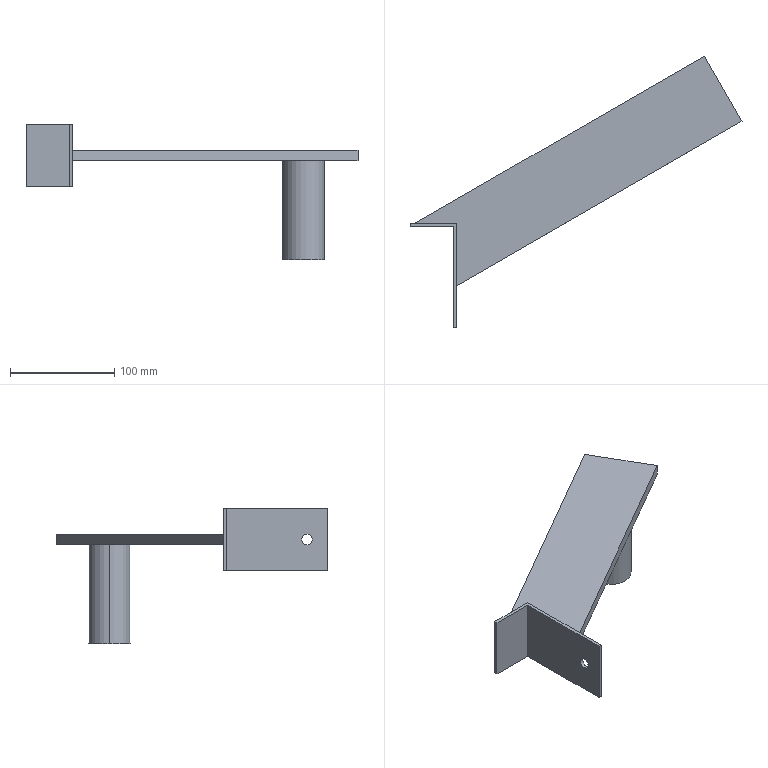Part | STEP file | 1 solid | 18 faces | box 318.145 x 260.315 x 130 mm | volume 361674 mm3 | plane 14 | cylinder 4 | commonest cylinder face diameters 10 x2 40 x2
STEP:
#1=CARTESIAN_POINT('',(0.,0.,0.));
#2=DIRECTION('',(0.,0.,1.));
#3=DIRECTION('',(1.,0.,0.));
#4=AXIS2_PLACEMENT_3D('',#1,#2,#3);
#5=CARTESIAN_POINT('',(51.255,-50.39,5.));
#6=VERTEX_POINT('',#5);
#7=CARTESIAN_POINT('',(48.255,-50.39,5.));
#8=VERTEX_POINT('',#7);
#9=CARTESIAN_POINT('',(51.255,-50.39,5.));
#10=DIRECTION('',(-1.,0.,0.));
#11=VECTOR('',#10,1.);
#12=LINE('',#9,#11);
#13=CARTESIAN_POINT('',(51.255,-50.39,0.));
#14=DIRECTION('',(-1.,0.,0.));
#15=DIRECTION('',(0.,0.,1.));
#16=AXIS2_PLACEMENT_3D('',#13,#14,#15);
#17=CYLINDRICAL_SURFACE('',#16,5.);
#18=CARTESIAN_POINT('',(6.283,0.));
#19=DIRECTION('',(0.,1.));
#20=VECTOR('',#19,1.);
#21=LINE('',#18,#20);
#22=(GEOMETRIC_REPRESENTATION_CONTEXT(2)PARAMETRIC_REPRESENTATION_CONTEXT()REPRESENTATION_CONTEXT('',''));
#23=DEFINITIONAL_REPRESENTATION('',(#21),#22);
#24=PCURVE('',#17,#23);
#25=CARTESIAN_POINT('',(51.255,-50.39,0.));
#26=DIRECTION('',(-1.,0.,0.));
#27=DIRECTION('',(0.,0.,1.));
#28=AXIS2_PLACEMENT_3D('',#25,#26,#27);
#29=CYLINDRICAL_SURFACE('',#28,5.);
#30=CARTESIAN_POINT('',(0.,0.));
#31=DIRECTION('',(0.,1.));
#32=VECTOR('',#31,1.);
#33=LINE('',#30,#32);
#34=(GEOMETRIC_REPRESENTATION_CONTEXT(2)PARAMETRIC_REPRESENTATION_CONTEXT()REPRESENTATION_CONTEXT('',''));
#35=DEFINITIONAL_REPRESENTATION('',(#33),#34);
#36=PCURVE('',#29,#35);
#37=SURFACE_CURVE('',#12,(#24,#36),.PCURVE_S1.);
#38=EDGE_CURVE('',#6,#8,#37,.T.);
#39=ORIENTED_EDGE('',*,*,#38,.T.);
#40=CARTESIAN_POINT('',(48.255,-50.39,-5.));
#41=VERTEX_POINT('',#40);
#42=CARTESIAN_POINT('',(48.255,-50.39,0.));
#43=DIRECTION('',(1.,0.,0.));
#44=DIRECTION('',(0.,0.,1.));
#45=AXIS2_PLACEMENT_3D('',#42,#43,#44);
#46=CIRCLE('',#45,5.);
#47=CARTESIAN_POINT('',(6.283,3.));
#48=DIRECTION('',(-1.,0.));
#49=VECTOR('',#48,1.);
#50=LINE('',#47,#49);
#51=(GEOMETRIC_REPRESENTATION_CONTEXT(2)PARAMETRIC_REPRESENTATION_CONTEXT()REPRESENTATION_CONTEXT('',''));
#52=DEFINITIONAL_REPRESENTATION('',(#50),#51);
#53=PCURVE('',#17,#52);
#54=CARTESIAN_POINT('',(48.255,26.61,0.));
#55=DIRECTION('',(1.,0.,0.));
#56=DIRECTION('',(0.,1.,0.));
#57=AXIS2_PLACEMENT_3D('',#54,#55,#56);
#58=PLANE('',#57);
#59=CARTESIAN_POINT('',(-77.,0.));
#60=DIRECTION('',(0.,1.));
#61=AXIS2_PLACEMENT_2D('',#59,#60);
#62=CIRCLE('',#61,5.);
#63=(GEOMETRIC_REPRESENTATION_CONTEXT(2)PARAMETRIC_REPRESENTATION_CONTEXT()REPRESENTATION_CONTEXT('',''));
#64=DEFINITIONAL_REPRESENTATION('',(#62),#63);
#65=PCURVE('',#58,#64);
#66=SURFACE_CURVE('',#46,(#53,#65),.PCURVE_S1.);
#67=EDGE_CURVE('',#8,#41,#66,.T.);
#68=ORIENTED_EDGE('',*,*,#67,.T.);
#69=CARTESIAN_POINT('',(51.255,-50.39,-5.));
#70=VERTEX_POINT('',#69);
#71=CARTESIAN_POINT('',(51.255,-50.39,-5.));
#72=DIRECTION('',(-1.,0.,0.));
#73=VECTOR('',#72,1.);
#74=LINE('',#71,#73);
#75=CARTESIAN_POINT('',(3.142,0.));
#76=DIRECTION('',(0.,1.));
#77=VECTOR('',#76,1.);
#78=LINE('',#75,#77);
#79=(GEOMETRIC_REPRESENTATION_CONTEXT(2)PARAMETRIC_REPRESENTATION_CONTEXT()REPRESENTATION_CONTEXT('',''));
#80=DEFINITIONAL_REPRESENTATION('',(#78),#79);
#81=PCURVE('',#17,#80);
#82=CARTESIAN_POINT('',(3.142,0.));
#83=DIRECTION('',(0.,1.));
#84=VECTOR('',#83,1.);
#85=LINE('',#82,#84);
#86=(GEOMETRIC_REPRESENTATION_CONTEXT(2)PARAMETRIC_REPRESENTATION_CONTEXT()REPRESENTATION_CONTEXT('',''));
#87=DEFINITIONAL_REPRESENTATION('',(#85),#86);
#88=PCURVE('',#29,#87);
#89=SURFACE_CURVE('',#74,(#81,#88),.PCURVE_S1.);
#90=EDGE_CURVE('',#70,#41,#89,.T.);
#91=ORIENTED_EDGE('',*,*,#90,.F.);
#92=CARTESIAN_POINT('',(51.255,-50.39,0.));
#93=DIRECTION('',(1.,0.,0.));
#94=DIRECTION('',(0.,0.,1.));
#95=AXIS2_PLACEMENT_3D('',#92,#93,#94);
#96=CIRCLE('',#95,5.);
#97=CARTESIAN_POINT('',(6.283,0.));
#98=DIRECTION('',(-1.,0.));
#99=VECTOR('',#98,1.);
#100=LINE('',#97,#99);
#101=(GEOMETRIC_REPRESENTATION_CONTEXT(2)PARAMETRIC_REPRESENTATION_CONTEXT()REPRESENTATION_CONTEXT('',''));
#102=DEFINITIONAL_REPRESENTATION('',(#100),#101);
#103=PCURVE('',#17,#102);
#104=CARTESIAN_POINT('',(51.255,-30.39,0.));
#105=DIRECTION('',(-1.,0.,0.));
#106=DIRECTION('',(0.,0.,1.));
#107=AXIS2_PLACEMENT_3D('',#104,#105,#106);
#108=PLANE('',#107);
#109=CARTESIAN_POINT('',(5.,-20.));
#110=CARTESIAN_POINT('',(5.,-28.66));
#111=CARTESIAN_POINT('',(-2.5,-24.33));
#112=CARTESIAN_POINT('',(-10.,-20.));
#113=CARTESIAN_POINT('',(-2.5,-15.67));
#114=CARTESIAN_POINT('',(5.,-11.34));
#115=CARTESIAN_POINT('',(5.,-20.));
#116=(BOUNDED_CURVE()B_SPLINE_CURVE(2,(#109,#110,#111,#112,#113,#114,#115),.UNSPECIFIED.,.T.,.F.)B_SPLINE_CURVE_WITH_KNOTS((1,2,2,2,2,1),(-2.094,0.,2.094,4.189,6.283,8.378),.UNSPECIFIED.)CURVE()GEOMETRIC_REPRESENTATION_ITEM()RATIONAL_B_SPLINE_CURVE((1.,0.5,1.,0.5,1.,0.5,1.))REPRESENTATION_ITEM(''));
#117=(GEOMETRIC_REPRESENTATION_CONTEXT(2)PARAMETRIC_REPRESENTATION_CONTEXT()REPRESENTATION_CONTEXT('',''));
#118=DEFINITIONAL_REPRESENTATION('',(#116),#117);
#119=PCURVE('',#108,#118);
#120=SURFACE_CURVE('',#96,(#103,#119),.PCURVE_S1.);
#121=EDGE_CURVE('',#6,#70,#120,.T.);
#122=ORIENTED_EDGE('',*,*,#121,.F.);
#123=EDGE_LOOP('',(#39,#68,#91,#122));
#124=FACE_BOUND('',#123,.F.);
#125=ADVANCED_FACE('',(#124),#17,.F.);
#126=CARTESIAN_POINT('',(252.733,139.027,-5.));
#127=VERTEX_POINT('',#126);
#128=CARTESIAN_POINT('',(292.733,139.027,-5.));
#129=VERTEX_POINT('',#128);
#130=CARTESIAN_POINT('',(272.733,139.027,-5.));
#131=DIRECTION('',(0.,0.,-1.));
#132=DIRECTION('',(-1.,0.,0.));
#133=AXIS2_PLACEMENT_3D('',#130,#131,#132);
#134=CIRCLE('',#133,20.);
#135=CARTESIAN_POINT('',(272.733,139.027,-5.));
#136=DIRECTION('',(0.,0.,-1.));
#137=DIRECTION('',(-1.,0.,0.));
#138=AXIS2_PLACEMENT_3D('',#135,#136,#137);
#139=CYLINDRICAL_SURFACE('',#138,20.);
#140=CARTESIAN_POINT('',(0.,0.));
#141=DIRECTION('',(1.,0.));
#142=VECTOR('',#141,1.);
#143=LINE('',#140,#142);
#144=(GEOMETRIC_REPRESENTATION_CONTEXT(2)PARAMETRIC_REPRESENTATION_CONTEXT()REPRESENTATION_CONTEXT('',''));
#145=DEFINITIONAL_REPRESENTATION('',(#143),#144);
#146=PCURVE('',#139,#145);
#147=CARTESIAN_POINT('',(244.528,123.338,-5.));
#148=DIRECTION('',(0.,0.,1.));
#149=DIRECTION('',(1.,0.,0.));
#150=AXIS2_PLACEMENT_3D('',#147,#148,#149);
#151=PLANE('',#150);
#152=CARTESIAN_POINT('',(8.205,15.689));
#153=CARTESIAN_POINT('',(8.205,50.33));
#154=CARTESIAN_POINT('',(38.205,33.01));
#155=CARTESIAN_POINT('',(68.205,15.689));
#156=CARTESIAN_POINT('',(38.205,-1.631));
#157=CARTESIAN_POINT('',(8.205,-18.952));
#158=CARTESIAN_POINT('',(8.205,15.689));
#159=(BOUNDED_CURVE()B_SPLINE_CURVE(2,(#152,#153,#154,#155,#156,#157,#158),.UNSPECIFIED.,.T.,.F.)B_SPLINE_CURVE_WITH_KNOTS((1,2,2,2,2,1),(-2.094,0.,2.094,4.189,6.283,8.378),.UNSPECIFIED.)CURVE()GEOMETRIC_REPRESENTATION_ITEM()RATIONAL_B_SPLINE_CURVE((1.,0.5,1.,0.5,1.,0.5,1.))REPRESENTATION_ITEM(''));
#160=(GEOMETRIC_REPRESENTATION_CONTEXT(2)PARAMETRIC_REPRESENTATION_CONTEXT()REPRESENTATION_CONTEXT('',''));
#161=DEFINITIONAL_REPRESENTATION('',(#159),#160);
#162=PCURVE('',#151,#161);
#163=SURFACE_CURVE('',#134,(#146,#162),.PCURVE_S1.);
#164=EDGE_CURVE('',#127,#129,#163,.T.);
#165=ORIENTED_EDGE('',*,*,#164,.T.);
#166=CARTESIAN_POINT('',(292.733,139.027,-100.));
#167=VERTEX_POINT('',#166);
#168=CARTESIAN_POINT('',(292.733,139.027,-5.));
#169=DIRECTION('',(0.,0.,-1.));
#170=VECTOR('',#169,1.);
#171=LINE('',#168,#170);
#172=CARTESIAN_POINT('',(3.142,0.));
#173=DIRECTION('',(0.,1.));
#174=VECTOR('',#173,1.);
#175=LINE('',#172,#174);
#176=(GEOMETRIC_REPRESENTATION_CONTEXT(2)PARAMETRIC_REPRESENTATION_CONTEXT()REPRESENTATION_CONTEXT('',''));
#177=DEFINITIONAL_REPRESENTATION('',(#175),#176);
#178=PCURVE('',#139,#177);
#179=CARTESIAN_POINT('',(272.733,139.027,-5.));
#180=DIRECTION('',(0.,0.,-1.));
#181=DIRECTION('',(-1.,0.,0.));
#182=AXIS2_PLACEMENT_3D('',#179,#180,#181);
#183=CYLINDRICAL_SURFACE('',#182,20.);
#184=CARTESIAN_POINT('',(3.142,0.));
#185=DIRECTION('',(0.,1.));
#186=VECTOR('',#185,1.);
#187=LINE('',#184,#186);
#188=(GEOMETRIC_REPRESENTATION_CONTEXT(2)PARAMETRIC_REPRESENTATION_CONTEXT()REPRESENTATION_CONTEXT('',''));
#189=DEFINITIONAL_REPRESENTATION('',(#187),#188);
#190=PCURVE('',#183,#189);
#191=SURFACE_CURVE('',#171,(#178,#190),.PCURVE_S1.);
#192=EDGE_CURVE('',#129,#167,#191,.T.);
#193=ORIENTED_EDGE('',*,*,#192,.T.);
#194=CARTESIAN_POINT('',(252.733,139.027,-100.));
#195=VERTEX_POINT('',#194);
#196=CARTESIAN_POINT('',(272.733,139.027,-100.));
#197=DIRECTION('',(0.,0.,1.));
#198=DIRECTION('',(-1.,0.,0.));
#199=AXIS2_PLACEMENT_3D('',#196,#197,#198);
#200=CIRCLE('',#199,20.);
#201=CARTESIAN_POINT('',(6.283,95.));
#202=DIRECTION('',(-1.,0.));
#203=VECTOR('',#202,1.);
#204=LINE('',#201,#203);
#205=(GEOMETRIC_REPRESENTATION_CONTEXT(2)PARAMETRIC_REPRESENTATION_CONTEXT()REPRESENTATION_CONTEXT('',''));
#206=DEFINITIONAL_REPRESENTATION('',(#204),#205);
#207=PCURVE('',#139,#206);
#208=CARTESIAN_POINT('',(272.733,139.027,-100.));
#209=DIRECTION('',(0.,0.,1.));
#210=DIRECTION('',(1.,0.,0.));
#211=AXIS2_PLACEMENT_3D('',#208,#209,#210);
#212=PLANE('',#211);
#213=CARTESIAN_POINT('',(0.,0.));
#214=DIRECTION('',(-1.,0.));
#215=AXIS2_PLACEMENT_2D('',#213,#214);
#216=CIRCLE('',#215,20.);
#217=(GEOMETRIC_REPRESENTATION_CONTEXT(2)PARAMETRIC_REPRESENTATION_CONTEXT()REPRESENTATION_CONTEXT('',''));
#218=DEFINITIONAL_REPRESENTATION('',(#216),#217);
#219=PCURVE('',#212,#218);
#220=SURFACE_CURVE('',#200,(#207,#219),.PCURVE_S1.);
#221=EDGE_CURVE('',#167,#195,#220,.T.);
#222=ORIENTED_EDGE('',*,*,#221,.T.);
#223=CARTESIAN_POINT('',(252.733,139.027,-5.));
#224=DIRECTION('',(0.,0.,-1.));
#225=VECTOR('',#224,1.);
#226=LINE('',#223,#225);
#227=CARTESIAN_POINT('',(0.,0.));
#228=DIRECTION('',(0.,1.));
#229=VECTOR('',#228,1.);
#230=LINE('',#227,#229);
#231=(GEOMETRIC_REPRESENTATION_CONTEXT(2)PARAMETRIC_REPRESENTATION_CONTEXT()REPRESENTATION_CONTEXT('',''));
#232=DEFINITIONAL_REPRESENTATION('',(#230),#231);
#233=PCURVE('',#139,#232);
#234=CARTESIAN_POINT('',(6.283,0.));
#235=DIRECTION('',(0.,1.));
#236=VECTOR('',#235,1.);
#237=LINE('',#234,#236);
#238=(GEOMETRIC_REPRESENTATION_CONTEXT(2)PARAMETRIC_REPRESENTATION_CONTEXT()REPRESENTATION_CONTEXT('',''));
#239=DEFINITIONAL_REPRESENTATION('',(#237),#238);
#240=PCURVE('',#183,#239);
#241=SURFACE_CURVE('',#226,(#233,#240),.PCURVE_S1.);
#242=EDGE_CURVE('',#127,#195,#241,.T.);
#243=ORIENTED_EDGE('',*,*,#242,.F.);
#244=EDGE_LOOP('',(#165,#193,#222,#243));
#245=FACE_BOUND('',#244,.T.);
#246=ADVANCED_FACE('',(#245),#139,.T.);
#247=CARTESIAN_POINT('',(11.255,29.61,5.));
#248=VERTEX_POINT('',#247);
#249=CARTESIAN_POINT('',(288.929,189.925,5.));
#250=VERTEX_POINT('',#249);
#251=CARTESIAN_POINT('',(11.255,29.61,5.));
#252=DIRECTION('',(0.866,0.5,0.));
#253=VECTOR('',#252,1.);
#254=LINE('',#251,#253);
#255=CARTESIAN_POINT('',(244.528,123.338,5.));
#256=DIRECTION('',(0.,0.,-1.));
#257=DIRECTION('',(-1.,0.,0.));
#258=AXIS2_PLACEMENT_3D('',#255,#256,#257);
#259=PLANE('',#258);
#260=CARTESIAN_POINT('',(233.273,-93.728));
#261=DIRECTION('',(-0.866,0.5));
#262=VECTOR('',#261,1.);
#263=LINE('',#260,#262);
#264=(GEOMETRIC_REPRESENTATION_CONTEXT(2)PARAMETRIC_REPRESENTATION_CONTEXT()REPRESENTATION_CONTEXT('',''));
#265=DEFINITIONAL_REPRESENTATION('',(#263),#264);
#266=PCURVE('',#259,#265);
#267=CARTESIAN_POINT('',(448.287,281.931,0.));
#268=DIRECTION('',(0.5,-0.866,0.));
#269=DIRECTION('',(0.866,0.5,0.));
#270=AXIS2_PLACEMENT_3D('',#267,#268,#269);
#271=PLANE('',#270);
#272=CARTESIAN_POINT('',(-504.641,5.));
#273=DIRECTION('',(1.,0.));
#274=VECTOR('',#273,1.);
#275=LINE('',#272,#274);
#276=(GEOMETRIC_REPRESENTATION_CONTEXT(2)PARAMETRIC_REPRESENTATION_CONTEXT()REPRESENTATION_CONTEXT('',''));
#277=DEFINITIONAL_REPRESENTATION('',(#275),#276);
#278=PCURVE('',#271,#277);
#279=SURFACE_CURVE('',#254,(#266,#278),.PCURVE_S1.);
#280=EDGE_CURVE('',#248,#250,#279,.T.);
#281=ORIENTED_EDGE('',*,*,#280,.F.);
#282=CARTESIAN_POINT('',(51.255,29.61,5.));
#283=VERTEX_POINT('',#282);
#284=CARTESIAN_POINT('',(244.528,29.61,5.));
#285=DIRECTION('',(-1.,0.,0.));
#286=VECTOR('',#285,1.);
#287=LINE('',#284,#286);
#288=CARTESIAN_POINT('',(0.,-93.728));
#289=DIRECTION('',(1.,0.));
#290=VECTOR('',#289,1.);
#291=LINE('',#288,#290);
#292=(GEOMETRIC_REPRESENTATION_CONTEXT(2)PARAMETRIC_REPRESENTATION_CONTEXT()REPRESENTATION_CONTEXT('',''));
#293=DEFINITIONAL_REPRESENTATION('',(#291),#292);
#294=PCURVE('',#259,#293);
#295=CARTESIAN_POINT('',(51.255,29.61,0.));
#296=DIRECTION('',(0.,-1.,0.));
#297=DIRECTION('',(0.,0.,-1.));
#298=AXIS2_PLACEMENT_3D('',#295,#296,#297);
#299=PLANE('',#298);
#300=CARTESIAN_POINT('',(-5.,193.273));
#301=DIRECTION('',(0.,-1.));
#302=VECTOR('',#301,1.);
#303=LINE('',#300,#302);
#304=(GEOMETRIC_REPRESENTATION_CONTEXT(2)PARAMETRIC_REPRESENTATION_CONTEXT()REPRESENTATION_CONTEXT('',''));
#305=DEFINITIONAL_REPRESENTATION('',(#303),#304);
#306=PCURVE('',#299,#305);
#307=SURFACE_CURVE('',#287,(#294,#306),.PCURVE_S1.);
#308=EDGE_CURVE('',#283,#248,#307,.T.);
#309=ORIENTED_EDGE('',*,*,#308,.F.);
#310=CARTESIAN_POINT('',(51.255,-30.39,5.));
#311=VERTEX_POINT('',#310);
#312=CARTESIAN_POINT('',(51.255,123.338,5.));
#313=DIRECTION('',(0.,1.,0.));
#314=VECTOR('',#313,1.);
#315=LINE('',#312,#314);
#316=CARTESIAN_POINT('',(193.273,0.));
#317=DIRECTION('',(0.,1.));
#318=VECTOR('',#317,1.);
#319=LINE('',#316,#318);
#320=(GEOMETRIC_REPRESENTATION_CONTEXT(2)PARAMETRIC_REPRESENTATION_CONTEXT()REPRESENTATION_CONTEXT('',''));
#321=DEFINITIONAL_REPRESENTATION('',(#319),#320);
#322=PCURVE('',#259,#321);
#323=CARTESIAN_POINT('',(5.,153.728));
#324=DIRECTION('',(0.,1.));
#325=VECTOR('',#324,1.);
#326=LINE('',#323,#325);
#327=(GEOMETRIC_REPRESENTATION_CONTEXT(2)PARAMETRIC_REPRESENTATION_CONTEXT()REPRESENTATION_CONTEXT('',''));
#328=DEFINITIONAL_REPRESENTATION('',(#326),#327);
#329=PCURVE('',#108,#328);
#330=SURFACE_CURVE('',#315,(#322,#329),.PCURVE_S1.);
#331=EDGE_CURVE('',#311,#283,#330,.T.);
#332=ORIENTED_EDGE('',*,*,#331,.F.);
#333=CARTESIAN_POINT('',(324.91,127.605,5.));
#334=VERTEX_POINT('',#333);
#335=CARTESIAN_POINT('',(324.91,127.605,5.));
#336=DIRECTION('',(-0.866,-0.5,0.));
#337=VECTOR('',#336,1.);
#338=LINE('',#335,#337);
#339=CARTESIAN_POINT('',(-80.382,4.267));
#340=DIRECTION('',(0.866,-0.5));
#341=VECTOR('',#340,1.);
#342=LINE('',#339,#341);
#343=(GEOMETRIC_REPRESENTATION_CONTEXT(2)PARAMETRIC_REPRESENTATION_CONTEXT()REPRESENTATION_CONTEXT('',''));
#344=DEFINITIONAL_REPRESENTATION('',(#342),#343);
#345=PCURVE('',#259,#344);
#346=CARTESIAN_POINT('',(51.255,-30.39,0.));
#347=DIRECTION('',(-0.5,0.866,0.));
#348=DIRECTION('',(-0.866,-0.5,0.));
#349=AXIS2_PLACEMENT_3D('',#346,#347,#348);
#350=PLANE('',#349);
#351=CARTESIAN_POINT('',(-315.989,5.));
#352=DIRECTION('',(1.,0.));
#353=VECTOR('',#352,1.);
#354=LINE('',#351,#353);
#355=(GEOMETRIC_REPRESENTATION_CONTEXT(2)PARAMETRIC_REPRESENTATION_CONTEXT()REPRESENTATION_CONTEXT('',''));
#356=DEFINITIONAL_REPRESENTATION('',(#354),#355);
#357=PCURVE('',#350,#356);
#358=SURFACE_CURVE('',#338,(#345,#357),.PCURVE_S1.);
#359=EDGE_CURVE('',#334,#311,#358,.T.);
#360=ORIENTED_EDGE('',*,*,#359,.F.);
#361=CARTESIAN_POINT('',(288.929,189.925,5.));
#362=DIRECTION('',(0.5,-0.866,0.));
#363=VECTOR('',#362,1.);
#364=LINE('',#361,#363);
#365=CARTESIAN_POINT('',(-44.401,66.587));
#366=DIRECTION('',(-0.5,-0.866));
#367=VECTOR('',#366,1.);
#368=LINE('',#365,#367);
#369=(GEOMETRIC_REPRESENTATION_CONTEXT(2)PARAMETRIC_REPRESENTATION_CONTEXT()REPRESENTATION_CONTEXT('',''));
#370=DEFINITIONAL_REPRESENTATION('',(#368),#369);
#371=PCURVE('',#259,#370);
#372=CARTESIAN_POINT('',(324.91,127.605,5.));
#373=DIRECTION('',(-0.866,-0.5,0.));
#374=DIRECTION('',(0.5,-0.866,0.));
#375=AXIS2_PLACEMENT_3D('',#372,#373,#374);
#376=PLANE('',#375);
#377=CARTESIAN_POINT('',(-71.962,0.));
#378=DIRECTION('',(1.,0.));
#379=VECTOR('',#378,1.);
#380=LINE('',#377,#379);
#381=(GEOMETRIC_REPRESENTATION_CONTEXT(2)PARAMETRIC_REPRESENTATION_CONTEXT()REPRESENTATION_CONTEXT('',''));
#382=DEFINITIONAL_REPRESENTATION('',(#380),#381);
#383=PCURVE('',#376,#382);
#384=SURFACE_CURVE('',#364,(#371,#383),.PCURVE_S1.);
#385=EDGE_CURVE('',#250,#334,#384,.T.);
#386=ORIENTED_EDGE('',*,*,#385,.F.);
#387=EDGE_LOOP('',(#281,#309,#332,#360,#386));
#388=FACE_BOUND('',#387,.T.);
#389=ADVANCED_FACE('',(#388),#259,.F.);
#390=CARTESIAN_POINT('',(288.929,189.925,-5.));
#391=VERTEX_POINT('',#390);
#392=CARTESIAN_POINT('',(288.929,189.925,5.));
#393=DIRECTION('',(0.,0.,-1.));
#394=VECTOR('',#393,1.);
#395=LINE('',#392,#394);
#396=CARTESIAN_POINT('',(-71.962,0.));
#397=DIRECTION('',(0.,-1.));
#398=VECTOR('',#397,1.);
#399=LINE('',#396,#398);
#400=(GEOMETRIC_REPRESENTATION_CONTEXT(2)PARAMETRIC_REPRESENTATION_CONTEXT()REPRESENTATION_CONTEXT('',''));
#401=DEFINITIONAL_REPRESENTATION('',(#399),#400);
#402=PCURVE('',#376,#401);
#403=CARTESIAN_POINT('',(-184.011,5.));
#404=DIRECTION('',(0.,-1.));
#405=VECTOR('',#404,1.);
#406=LINE('',#403,#405);
#407=(GEOMETRIC_REPRESENTATION_CONTEXT(2)PARAMETRIC_REPRESENTATION_CONTEXT()REPRESENTATION_CONTEXT('',''));
#408=DEFINITIONAL_REPRESENTATION('',(#406),#407);
#409=PCURVE('',#271,#408);
#410=SURFACE_CURVE('',#395,(#402,#409),.PCURVE_S1.);
#411=EDGE_CURVE('',#250,#391,#410,.T.);
#412=ORIENTED_EDGE('',*,*,#411,.F.);
#413=ORIENTED_EDGE('',*,*,#385,.T.);
#414=CARTESIAN_POINT('',(324.91,127.605,-5.));
#415=VERTEX_POINT('',#414);
#416=CARTESIAN_POINT('',(324.91,127.605,5.));
#417=DIRECTION('',(0.,0.,1.));
#418=VECTOR('',#417,1.);
#419=LINE('',#416,#418);
#420=CARTESIAN_POINT('',(0.,0.));
#421=DIRECTION('',(0.,1.));
#422=VECTOR('',#421,1.);
#423=LINE('',#420,#422);
#424=(GEOMETRIC_REPRESENTATION_CONTEXT(2)PARAMETRIC_REPRESENTATION_CONTEXT()REPRESENTATION_CONTEXT('',''));
#425=DEFINITIONAL_REPRESENTATION('',(#423),#424);
#426=PCURVE('',#376,#425);
#427=CARTESIAN_POINT('',(-315.989,5.));
#428=DIRECTION('',(0.,1.));
#429=VECTOR('',#428,1.);
#430=LINE('',#427,#429);
#431=(GEOMETRIC_REPRESENTATION_CONTEXT(2)PARAMETRIC_REPRESENTATION_CONTEXT()REPRESENTATION_CONTEXT('',''));
#432=DEFINITIONAL_REPRESENTATION('',(#430),#431);
#433=PCURVE('',#350,#432);
#434=SURFACE_CURVE('',#419,(#426,#433),.PCURVE_S1.);
#435=EDGE_CURVE('',#415,#334,#434,.T.);
#436=ORIENTED_EDGE('',*,*,#435,.F.);
#437=CARTESIAN_POINT('',(324.91,127.605,-5.));
#438=DIRECTION('',(0.5,-0.866,0.));
#439=VECTOR('',#438,1.);
#440=LINE('',#437,#439);
#441=CARTESIAN_POINT('',(0.,-10.));
#442=DIRECTION('',(1.,0.));
#443=VECTOR('',#442,1.);
#444=LINE('',#441,#443);
#445=(GEOMETRIC_REPRESENTATION_CONTEXT(2)PARAMETRIC_REPRESENTATION_CONTEXT()REPRESENTATION_CONTEXT('',''));
#446=DEFINITIONAL_REPRESENTATION('',(#444),#445);
#447=PCURVE('',#376,#446);
#448=CARTESIAN_POINT('',(80.382,4.267));
#449=DIRECTION('',(0.5,-0.866));
#450=VECTOR('',#449,1.);
#451=LINE('',#448,#450);
#452=(GEOMETRIC_REPRESENTATION_CONTEXT(2)PARAMETRIC_REPRESENTATION_CONTEXT()REPRESENTATION_CONTEXT('',''));
#453=DEFINITIONAL_REPRESENTATION('',(#451),#452);
#454=PCURVE('',#151,#453);
#455=SURFACE_CURVE('',#440,(#447,#454),.PCURVE_S1.);
#456=EDGE_CURVE('',#391,#415,#455,.T.);
#457=ORIENTED_EDGE('',*,*,#456,.F.);
#458=EDGE_LOOP('',(#412,#413,#436,#457));
#459=FACE_BOUND('',#458,.T.);
#460=ADVANCED_FACE('',(#459),#376,.F.);
#461=CARTESIAN_POINT('',(11.255,29.61,-5.));
#462=VERTEX_POINT('',#461);
#463=CARTESIAN_POINT('',(448.287,281.931,-5.));
#464=DIRECTION('',(0.866,0.5,0.));
#465=VECTOR('',#464,1.);
#466=LINE('',#463,#465);
#467=CARTESIAN_POINT('',(0.,-5.));
#468=DIRECTION('',(1.,0.));
#469=VECTOR('',#468,1.);
#470=LINE('',#467,#469);
#471=(GEOMETRIC_REPRESENTATION_CONTEXT(2)PARAMETRIC_REPRESENTATION_CONTEXT()REPRESENTATION_CONTEXT('',''));
#472=DEFINITIONAL_REPRESENTATION('',(#470),#471);
#473=PCURVE('',#271,#472);
#474=CARTESIAN_POINT('',(203.759,158.592));
#475=DIRECTION('',(0.866,0.5));
#476=VECTOR('',#475,1.);
#477=LINE('',#474,#476);
#478=(GEOMETRIC_REPRESENTATION_CONTEXT(2)PARAMETRIC_REPRESENTATION_CONTEXT()REPRESENTATION_CONTEXT('',''));
#479=DEFINITIONAL_REPRESENTATION('',(#477),#478);
#480=PCURVE('',#151,#479);
#481=SURFACE_CURVE('',#466,(#473,#480),.PCURVE_S1.);
#482=EDGE_CURVE('',#462,#391,#481,.T.);
#483=ORIENTED_EDGE('',*,*,#482,.F.);
#484=CARTESIAN_POINT('',(11.255,29.61,0.));
#485=DIRECTION('',(0.,0.,-1.));
#486=VECTOR('',#485,1.);
#487=LINE('',#484,#486);
#488=CARTESIAN_POINT('',(-504.641,0.));
#489=DIRECTION('',(0.,-1.));
#490=VECTOR('',#489,1.);
#491=LINE('',#488,#490);
#492=(GEOMETRIC_REPRESENTATION_CONTEXT(2)PARAMETRIC_REPRESENTATION_CONTEXT()REPRESENTATION_CONTEXT('',''));
#493=DEFINITIONAL_REPRESENTATION('',(#491),#492);
#494=PCURVE('',#271,#493);
#495=CARTESIAN_POINT('',(0.,-40.));
#496=DIRECTION('',(1.,0.));
#497=VECTOR('',#496,1.);
#498=LINE('',#495,#497);
#499=(GEOMETRIC_REPRESENTATION_CONTEXT(2)PARAMETRIC_REPRESENTATION_CONTEXT()REPRESENTATION_CONTEXT('',''));
#500=DEFINITIONAL_REPRESENTATION('',(#498),#499);
#501=PCURVE('',#299,#500);
#502=SURFACE_CURVE('',#487,(#494,#501),.PCURVE_S1.);
#503=EDGE_CURVE('',#248,#462,#502,.T.);
#504=ORIENTED_EDGE('',*,*,#503,.F.);
#505=ORIENTED_EDGE('',*,*,#280,.T.);
#506=ORIENTED_EDGE('',*,*,#411,.T.);
#507=EDGE_LOOP('',(#483,#504,#505,#506));
#508=FACE_BOUND('',#507,.T.);
#509=ADVANCED_FACE('',(#508),#271,.F.);
#510=CARTESIAN_POINT('',(51.255,29.61,30.));
#511=VERTEX_POINT('',#510);
#512=CARTESIAN_POINT('',(6.765,29.61,30.));
#513=VERTEX_POINT('',#512);
#514=CARTESIAN_POINT('',(51.255,29.61,30.));
#515=DIRECTION('',(-1.,0.,0.));
#516=VECTOR('',#515,1.);
#517=LINE('',#514,#516);
#518=CARTESIAN_POINT('',(-30.,0.));
#519=DIRECTION('',(0.,-1.));
#520=VECTOR('',#519,1.);
#521=LINE('',#518,#520);
#522=(GEOMETRIC_REPRESENTATION_CONTEXT(2)PARAMETRIC_REPRESENTATION_CONTEXT()REPRESENTATION_CONTEXT('',''));
#523=DEFINITIONAL_REPRESENTATION('',(#521),#522);
#524=PCURVE('',#299,#523);
#525=CARTESIAN_POINT('',(28.15,15.005,30.));
#526=DIRECTION('',(0.,0.,-1.));
#527=DIRECTION('',(-1.,0.,0.));
#528=AXIS2_PLACEMENT_3D('',#525,#526,#527);
#529=PLANE('',#528);
#530=CARTESIAN_POINT('',(-23.106,14.606));
#531=DIRECTION('',(1.,0.));
#532=VECTOR('',#531,1.);
#533=LINE('',#530,#532);
#534=(GEOMETRIC_REPRESENTATION_CONTEXT(2)PARAMETRIC_REPRESENTATION_CONTEXT()REPRESENTATION_CONTEXT('',''));
#535=DEFINITIONAL_REPRESENTATION('',(#533),#534);
#536=PCURVE('',#529,#535);
#537=SURFACE_CURVE('',#517,(#524,#536),.PCURVE_S1.);
#538=EDGE_CURVE('',#511,#513,#537,.T.);
#539=ORIENTED_EDGE('',*,*,#538,.F.);
#540=CARTESIAN_POINT('',(51.255,29.61,0.));
#541=DIRECTION('',(0.,0.,1.));
#542=VECTOR('',#541,1.);
#543=LINE('',#540,#542);
#544=CARTESIAN_POINT('',(0.,0.));
#545=DIRECTION('',(-1.,0.));
#546=VECTOR('',#545,1.);
#547=LINE('',#544,#546);
#548=(GEOMETRIC_REPRESENTATION_CONTEXT(2)PARAMETRIC_REPRESENTATION_CONTEXT()REPRESENTATION_CONTEXT('',''));
#549=DEFINITIONAL_REPRESENTATION('',(#547),#548);
#550=PCURVE('',#299,#549);
#551=CARTESIAN_POINT('',(0.,60.));
#552=DIRECTION('',(1.,0.));
#553=VECTOR('',#552,1.);
#554=LINE('',#551,#553);
#555=(GEOMETRIC_REPRESENTATION_CONTEXT(2)PARAMETRIC_REPRESENTATION_CONTEXT()REPRESENTATION_CONTEXT('',''));
#556=DEFINITIONAL_REPRESENTATION('',(#554),#555);
#557=PCURVE('',#108,#556);
#558=SURFACE_CURVE('',#543,(#550,#557),.PCURVE_S1.);
#559=EDGE_CURVE('',#283,#511,#558,.T.);
#560=ORIENTED_EDGE('',*,*,#559,.F.);
#561=ORIENTED_EDGE('',*,*,#308,.T.);
#562=ORIENTED_EDGE('',*,*,#503,.T.);
#563=CARTESIAN_POINT('',(51.255,29.61,-5.));
#564=VERTEX_POINT('',#563);
#565=CARTESIAN_POINT('',(51.255,29.61,-5.));
#566=DIRECTION('',(-1.,0.,0.));
#567=VECTOR('',#566,1.);
#568=LINE('',#565,#567);
#569=CARTESIAN_POINT('',(5.,0.));
#570=DIRECTION('',(0.,-1.));
#571=VECTOR('',#570,1.);
#572=LINE('',#569,#571);
#573=(GEOMETRIC_REPRESENTATION_CONTEXT(2)PARAMETRIC_REPRESENTATION_CONTEXT()REPRESENTATION_CONTEXT('',''));
#574=DEFINITIONAL_REPRESENTATION('',(#572),#573);
#575=PCURVE('',#299,#574);
#576=CARTESIAN_POINT('',(-193.273,-93.728));
#577=DIRECTION('',(-1.,0.));
#578=VECTOR('',#577,1.);
#579=LINE('',#576,#578);
#580=(GEOMETRIC_REPRESENTATION_CONTEXT(2)PARAMETRIC_REPRESENTATION_CONTEXT()REPRESENTATION_CONTEXT('',''));
#581=DEFINITIONAL_REPRESENTATION('',(#579),#580);
#582=PCURVE('',#151,#581);
#583=SURFACE_CURVE('',#568,(#575,#582),.PCURVE_S1.);
#584=EDGE_CURVE('',#564,#462,#583,.T.);
#585=ORIENTED_EDGE('',*,*,#584,.F.);
#586=CARTESIAN_POINT('',(51.255,29.61,-30.));
#587=VERTEX_POINT('',#586);
#588=CARTESIAN_POINT('',(51.255,29.61,0.));
#589=DIRECTION('',(0.,0.,1.));
#590=VECTOR('',#589,1.);
#591=LINE('',#588,#590);
#592=CARTESIAN_POINT('',(0.,0.));
#593=DIRECTION('',(-1.,0.));
#594=VECTOR('',#593,1.);
#595=LINE('',#592,#594);
#596=(GEOMETRIC_REPRESENTATION_CONTEXT(2)PARAMETRIC_REPRESENTATION_CONTEXT()REPRESENTATION_CONTEXT('',''));
#597=DEFINITIONAL_REPRESENTATION('',(#595),#596);
#598=PCURVE('',#299,#597);
#599=CARTESIAN_POINT('',(0.,60.));
#600=DIRECTION('',(1.,0.));
#601=VECTOR('',#600,1.);
#602=LINE('',#599,#601);
#603=(GEOMETRIC_REPRESENTATION_CONTEXT(2)PARAMETRIC_REPRESENTATION_CONTEXT()REPRESENTATION_CONTEXT('',''));
#604=DEFINITIONAL_REPRESENTATION('',(#602),#603);
#605=PCURVE('',#108,#604);
#606=SURFACE_CURVE('',#591,(#598,#605),.PCURVE_S1.);
#607=EDGE_CURVE('',#587,#564,#606,.T.);
#608=ORIENTED_EDGE('',*,*,#607,.F.);
#609=CARTESIAN_POINT('',(6.765,29.61,-30.));
#610=VERTEX_POINT('',#609);
#611=CARTESIAN_POINT('',(51.255,29.61,-30.));
#612=DIRECTION('',(1.,0.,0.));
#613=VECTOR('',#612,1.);
#614=LINE('',#611,#613);
#615=CARTESIAN_POINT('',(30.,0.));
#616=DIRECTION('',(0.,1.));
#617=VECTOR('',#616,1.);
#618=LINE('',#615,#617);
#619=(GEOMETRIC_REPRESENTATION_CONTEXT(2)PARAMETRIC_REPRESENTATION_CONTEXT()REPRESENTATION_CONTEXT('',''));
#620=DEFINITIONAL_REPRESENTATION('',(#618),#619);
#621=PCURVE('',#299,#620);
#622=CARTESIAN_POINT('',(28.15,15.005,-30.));
#623=DIRECTION('',(0.,0.,1.));
#624=DIRECTION('',(1.,0.,0.));
#625=AXIS2_PLACEMENT_3D('',#622,#623,#624);
#626=PLANE('',#625);
#627=CARTESIAN_POINT('',(23.106,14.606));
#628=DIRECTION('',(1.,0.));
#629=VECTOR('',#628,1.);
#630=LINE('',#627,#629);
#631=(GEOMETRIC_REPRESENTATION_CONTEXT(2)PARAMETRIC_REPRESENTATION_CONTEXT()REPRESENTATION_CONTEXT('',''));
#632=DEFINITIONAL_REPRESENTATION('',(#630),#631);
#633=PCURVE('',#626,#632);
#634=SURFACE_CURVE('',#614,(#621,#633),.PCURVE_S1.);
#635=EDGE_CURVE('',#610,#587,#634,.T.);
#636=ORIENTED_EDGE('',*,*,#635,.F.);
#637=CARTESIAN_POINT('',(6.765,29.61,0.));
#638=DIRECTION('',(0.,0.,-1.));
#639=VECTOR('',#638,1.);
#640=LINE('',#637,#639);
#641=CARTESIAN_POINT('',(0.,-44.49));
#642=DIRECTION('',(1.,0.));
#643=VECTOR('',#642,1.);
#644=LINE('',#641,#643);
#645=(GEOMETRIC_REPRESENTATION_CONTEXT(2)PARAMETRIC_REPRESENTATION_CONTEXT()REPRESENTATION_CONTEXT('',''));
#646=DEFINITIONAL_REPRESENTATION('',(#644),#645);
#647=PCURVE('',#299,#646);
#648=CARTESIAN_POINT('',(6.765,29.61,-30.));
#649=DIRECTION('',(1.,0.,0.));
#650=DIRECTION('',(0.,0.,-1.));
#651=AXIS2_PLACEMENT_3D('',#648,#649,#650);
#652=PLANE('',#651);
#653=CARTESIAN_POINT('',(-30.,0.));
#654=DIRECTION('',(1.,0.));
#655=VECTOR('',#654,1.);
#656=LINE('',#653,#655);
#657=(GEOMETRIC_REPRESENTATION_CONTEXT(2)PARAMETRIC_REPRESENTATION_CONTEXT()REPRESENTATION_CONTEXT('',''));
#658=DEFINITIONAL_REPRESENTATION('',(#656),#657);
#659=PCURVE('',#652,#658);
#660=SURFACE_CURVE('',#640,(#647,#659),.PCURVE_S1.);
#661=EDGE_CURVE('',#513,#610,#660,.T.);
#662=ORIENTED_EDGE('',*,*,#661,.F.);
#663=EDGE_LOOP('',(#539,#560,#561,#562,#585,#608,#636,#662));
#664=FACE_BOUND('',#663,.T.);
#665=ADVANCED_FACE('',(#664),#299,.F.);
#666=CARTESIAN_POINT('',(51.255,-30.39,-5.));
#667=VERTEX_POINT('',#666);
#668=CARTESIAN_POINT('',(51.255,-30.39,0.));
#669=DIRECTION('',(0.,0.,-1.));
#670=VECTOR('',#669,1.);
#671=LINE('',#668,#670);
#672=CARTESIAN_POINT('',(0.,0.));
#673=DIRECTION('',(-1.,0.));
#674=VECTOR('',#673,1.);
#675=LINE('',#672,#674);
#676=(GEOMETRIC_REPRESENTATION_CONTEXT(2)PARAMETRIC_REPRESENTATION_CONTEXT()REPRESENTATION_CONTEXT('',''));
#677=DEFINITIONAL_REPRESENTATION('',(#675),#676);
#678=PCURVE('',#108,#677);
#679=CARTESIAN_POINT('',(0.,0.));
#680=DIRECTION('',(0.,-1.));
#681=VECTOR('',#680,1.);
#682=LINE('',#679,#681);
#683=(GEOMETRIC_REPRESENTATION_CONTEXT(2)PARAMETRIC_REPRESENTATION_CONTEXT()REPRESENTATION_CONTEXT('',''));
#684=DEFINITIONAL_REPRESENTATION('',(#682),#683);
#685=PCURVE('',#350,#684);
#686=SURFACE_CURVE('',#671,(#678,#685),.PCURVE_S1.);
#687=EDGE_CURVE('',#311,#667,#686,.T.);
#688=ORIENTED_EDGE('',*,*,#687,.F.);
#689=ORIENTED_EDGE('',*,*,#331,.T.);
#690=ORIENTED_EDGE('',*,*,#559,.T.);
#691=CARTESIAN_POINT('',(51.255,-70.39,30.));
#692=VERTEX_POINT('',#691);
#693=CARTESIAN_POINT('',(51.255,-30.39,30.));
#694=DIRECTION('',(0.,1.,0.));
#695=VECTOR('',#694,1.);
#696=LINE('',#693,#695);
#697=CARTESIAN_POINT('',(30.,0.));
#698=DIRECTION('',(0.,1.));
#699=VECTOR('',#698,1.);
#700=LINE('',#697,#699);
#701=(GEOMETRIC_REPRESENTATION_CONTEXT(2)PARAMETRIC_REPRESENTATION_CONTEXT()REPRESENTATION_CONTEXT('',''));
#702=DEFINITIONAL_REPRESENTATION('',(#700),#701);
#703=PCURVE('',#108,#702);
#704=CARTESIAN_POINT('',(-23.106,-45.394));
#705=DIRECTION('',(0.,1.));
#706=VECTOR('',#705,1.);
#707=LINE('',#704,#706);
#708=(GEOMETRIC_REPRESENTATION_CONTEXT(2)PARAMETRIC_REPRESENTATION_CONTEXT()REPRESENTATION_CONTEXT('',''));
#709=DEFINITIONAL_REPRESENTATION('',(#707),#708);
#710=PCURVE('',#529,#709);
#711=SURFACE_CURVE('',#696,(#703,#710),.PCURVE_S1.);
#712=EDGE_CURVE('',#692,#511,#711,.T.);
#713=ORIENTED_EDGE('',*,*,#712,.F.);
#714=CARTESIAN_POINT('',(51.255,-70.39,-30.));
#715=VERTEX_POINT('',#714);
#716=CARTESIAN_POINT('',(51.255,-70.39,0.));
#717=DIRECTION('',(0.,0.,1.));
#718=VECTOR('',#717,1.);
#719=LINE('',#716,#718);
#720=CARTESIAN_POINT('',(0.,-40.));
#721=DIRECTION('',(1.,0.));
#722=VECTOR('',#721,1.);
#723=LINE('',#720,#722);
#724=(GEOMETRIC_REPRESENTATION_CONTEXT(2)PARAMETRIC_REPRESENTATION_CONTEXT()REPRESENTATION_CONTEXT('',''));
#725=DEFINITIONAL_REPRESENTATION('',(#723),#724);
#726=PCURVE('',#108,#725);
#727=CARTESIAN_POINT('',(49.755,-70.39,0.));
#728=DIRECTION('',(0.,-1.,0.));
#729=DIRECTION('',(0.,0.,-1.));
#730=AXIS2_PLACEMENT_3D('',#727,#728,#729);
#731=PLANE('',#730);
#732=CARTESIAN_POINT('',(0.,1.5));
#733=DIRECTION('',(-1.,0.));
#734=VECTOR('',#733,1.);
#735=LINE('',#732,#734);
#736=(GEOMETRIC_REPRESENTATION_CONTEXT(2)PARAMETRIC_REPRESENTATION_CONTEXT()REPRESENTATION_CONTEXT('',''));
#737=DEFINITIONAL_REPRESENTATION('',(#735),#736);
#738=PCURVE('',#731,#737);
#739=SURFACE_CURVE('',#719,(#726,#738),.PCURVE_S1.);
#740=EDGE_CURVE('',#715,#692,#739,.T.);
#741=ORIENTED_EDGE('',*,*,#740,.F.);
#742=CARTESIAN_POINT('',(51.255,-30.39,-30.));
#743=DIRECTION('',(0.,-1.,0.));
#744=VECTOR('',#743,1.);
#745=LINE('',#742,#744);
#746=CARTESIAN_POINT('',(-30.,0.));
#747=DIRECTION('',(0.,-1.));
#748=VECTOR('',#747,1.);
#749=LINE('',#746,#748);
#750=(GEOMETRIC_REPRESENTATION_CONTEXT(2)PARAMETRIC_REPRESENTATION_CONTEXT()REPRESENTATION_CONTEXT('',''));
#751=DEFINITIONAL_REPRESENTATION('',(#749),#750);
#752=PCURVE('',#108,#751);
#753=CARTESIAN_POINT('',(23.106,-45.394));
#754=DIRECTION('',(0.,-1.));
#755=VECTOR('',#754,1.);
#756=LINE('',#753,#755);
#757=(GEOMETRIC_REPRESENTATION_CONTEXT(2)PARAMETRIC_REPRESENTATION_CONTEXT()REPRESENTATION_CONTEXT('',''));
#758=DEFINITIONAL_REPRESENTATION('',(#756),#757);
#759=PCURVE('',#626,#758);
#760=SURFACE_CURVE('',#745,(#752,#759),.PCURVE_S1.);
#761=EDGE_CURVE('',#587,#715,#760,.T.);
#762=ORIENTED_EDGE('',*,*,#761,.F.);
#763=ORIENTED_EDGE('',*,*,#607,.T.);
#764=CARTESIAN_POINT('',(51.255,-30.39,-5.));
#765=DIRECTION('',(0.,1.,0.));
#766=VECTOR('',#765,1.);
#767=LINE('',#764,#766);
#768=CARTESIAN_POINT('',(-5.,0.));
#769=DIRECTION('',(0.,1.));
#770=VECTOR('',#769,1.);
#771=LINE('',#768,#770);
#772=(GEOMETRIC_REPRESENTATION_CONTEXT(2)PARAMETRIC_REPRESENTATION_CONTEXT()REPRESENTATION_CONTEXT('',''));
#773=DEFINITIONAL_REPRESENTATION('',(#771),#772);
#774=PCURVE('',#108,#773);
#775=CARTESIAN_POINT('',(-193.273,-153.728));
#776=DIRECTION('',(0.,1.));
#777=VECTOR('',#776,1.);
#778=LINE('',#775,#777);
#779=(GEOMETRIC_REPRESENTATION_CONTEXT(2)PARAMETRIC_REPRESENTATION_CONTEXT()REPRESENTATION_CONTEXT('',''));
#780=DEFINITIONAL_REPRESENTATION('',(#778),#779);
#781=PCURVE('',#151,#780);
#782=SURFACE_CURVE('',#767,(#774,#781),.PCURVE_S1.);
#783=EDGE_CURVE('',#667,#564,#782,.T.);
#784=ORIENTED_EDGE('',*,*,#783,.F.);
#785=EDGE_LOOP('',(#688,#689,#690,#713,#741,#762,#763,#784));
#786=FACE_BOUND('',#785,.T.);
#787=ORIENTED_EDGE('',*,*,#121,.F.);
#788=CARTESIAN_POINT('',(51.255,-50.39,0.));
#789=DIRECTION('',(1.,0.,0.));
#790=DIRECTION('',(0.,0.,1.));
#791=AXIS2_PLACEMENT_3D('',#788,#789,#790);
#792=CIRCLE('',#791,5.);
#793=CARTESIAN_POINT('',(5.,-20.));
#794=CARTESIAN_POINT('',(5.,-28.66));
#795=CARTESIAN_POINT('',(-2.5,-24.33));
#796=CARTESIAN_POINT('',(-10.,-20.));
#797=CARTESIAN_POINT('',(-2.5,-15.67));
#798=CARTESIAN_POINT('',(5.,-11.34));
#799=CARTESIAN_POINT('',(5.,-20.));
#800=(BOUNDED_CURVE()B_SPLINE_CURVE(2,(#793,#794,#795,#796,#797,#798,#799),.UNSPECIFIED.,.T.,.F.)B_SPLINE_CURVE_WITH_KNOTS((1,2,2,2,2,1),(-2.094,0.,2.094,4.189,6.283,8.378),.UNSPECIFIED.)CURVE()GEOMETRIC_REPRESENTATION_ITEM()RATIONAL_B_SPLINE_CURVE((1.,0.5,1.,0.5,1.,0.5,1.))REPRESENTATION_ITEM(''));
#801=(GEOMETRIC_REPRESENTATION_CONTEXT(2)PARAMETRIC_REPRESENTATION_CONTEXT()REPRESENTATION_CONTEXT('',''));
#802=DEFINITIONAL_REPRESENTATION('',(#800),#801);
#803=PCURVE('',#108,#802);
#804=CARTESIAN_POINT('',(6.283,0.));
#805=DIRECTION('',(-1.,0.));
#806=VECTOR('',#805,1.);
#807=LINE('',#804,#806);
#808=(GEOMETRIC_REPRESENTATION_CONTEXT(2)PARAMETRIC_REPRESENTATION_CONTEXT()REPRESENTATION_CONTEXT('',''));
#809=DEFINITIONAL_REPRESENTATION('',(#807),#808);
#810=PCURVE('',#29,#809);
#811=SURFACE_CURVE('',#792,(#803,#810),.PCURVE_S1.);
#812=EDGE_CURVE('',#70,#6,#811,.T.);
#813=ORIENTED_EDGE('',*,*,#812,.F.);
#814=EDGE_LOOP('',(#787,#813));
#815=FACE_BOUND('',#814,.T.);
#816=ADVANCED_FACE('',(#786,#815),#108,.F.);
#817=ORIENTED_EDGE('',*,*,#359,.T.);
#818=ORIENTED_EDGE('',*,*,#687,.T.);
#819=CARTESIAN_POINT('',(51.255,-30.39,-5.));
#820=DIRECTION('',(-0.866,-0.5,0.));
#821=VECTOR('',#820,1.);
#822=LINE('',#819,#821);
#823=CARTESIAN_POINT('',(0.,-5.));
#824=DIRECTION('',(1.,0.));
#825=VECTOR('',#824,1.);
#826=LINE('',#823,#825);
#827=(GEOMETRIC_REPRESENTATION_CONTEXT(2)PARAMETRIC_REPRESENTATION_CONTEXT()REPRESENTATION_CONTEXT('',''));
#828=DEFINITIONAL_REPRESENTATION('',(#826),#827);
#829=PCURVE('',#350,#828);
#830=CARTESIAN_POINT('',(-193.273,-153.728));
#831=DIRECTION('',(-0.866,-0.5));
#832=VECTOR('',#831,1.);
#833=LINE('',#830,#832);
#834=(GEOMETRIC_REPRESENTATION_CONTEXT(2)PARAMETRIC_REPRESENTATION_CONTEXT()REPRESENTATION_CONTEXT('',''));
#835=DEFINITIONAL_REPRESENTATION('',(#833),#834);
#836=PCURVE('',#151,#835);
#837=SURFACE_CURVE('',#822,(#829,#836),.PCURVE_S1.);
#838=EDGE_CURVE('',#415,#667,#837,.T.);
#839=ORIENTED_EDGE('',*,*,#838,.F.);
#840=ORIENTED_EDGE('',*,*,#435,.T.);
#841=EDGE_LOOP('',(#817,#818,#839,#840));
#842=FACE_BOUND('',#841,.T.);
#843=ADVANCED_FACE('',(#842),#350,.F.);
#844=ORIENTED_EDGE('',*,*,#838,.T.);
#845=ORIENTED_EDGE('',*,*,#783,.T.);
#846=ORIENTED_EDGE('',*,*,#584,.T.);
#847=ORIENTED_EDGE('',*,*,#482,.T.);
#848=ORIENTED_EDGE('',*,*,#456,.T.);
#849=EDGE_LOOP('',(#844,#845,#846,#847,#848));
#850=FACE_BOUND('',#849,.T.);
#851=ORIENTED_EDGE('',*,*,#164,.F.);
#852=CARTESIAN_POINT('',(272.733,139.027,-5.));
#853=DIRECTION('',(0.,0.,-1.));
#854=DIRECTION('',(-1.,0.,0.));
#855=AXIS2_PLACEMENT_3D('',#852,#853,#854);
#856=CIRCLE('',#855,20.);
#857=CARTESIAN_POINT('',(8.205,15.689));
#858=CARTESIAN_POINT('',(8.205,50.33));
#859=CARTESIAN_POINT('',(38.205,33.01));
#860=CARTESIAN_POINT('',(68.205,15.689));
#861=CARTESIAN_POINT('',(38.205,-1.631));
#862=CARTESIAN_POINT('',(8.205,-18.952));
#863=CARTESIAN_POINT('',(8.205,15.689));
#864=(BOUNDED_CURVE()B_SPLINE_CURVE(2,(#857,#858,#859,#860,#861,#862,#863),.UNSPECIFIED.,.T.,.F.)B_SPLINE_CURVE_WITH_KNOTS((1,2,2,2,2,1),(-2.094,0.,2.094,4.189,6.283,8.378),.UNSPECIFIED.)CURVE()GEOMETRIC_REPRESENTATION_ITEM()RATIONAL_B_SPLINE_CURVE((1.,0.5,1.,0.5,1.,0.5,1.))REPRESENTATION_ITEM(''));
#865=(GEOMETRIC_REPRESENTATION_CONTEXT(2)PARAMETRIC_REPRESENTATION_CONTEXT()REPRESENTATION_CONTEXT('',''));
#866=DEFINITIONAL_REPRESENTATION('',(#864),#865);
#867=PCURVE('',#151,#866);
#868=CARTESIAN_POINT('',(0.,0.));
#869=DIRECTION('',(1.,0.));
#870=VECTOR('',#869,1.);
#871=LINE('',#868,#870);
#872=(GEOMETRIC_REPRESENTATION_CONTEXT(2)PARAMETRIC_REPRESENTATION_CONTEXT()REPRESENTATION_CONTEXT('',''));
#873=DEFINITIONAL_REPRESENTATION('',(#871),#872);
#874=PCURVE('',#183,#873);
#875=SURFACE_CURVE('',#856,(#867,#874),.PCURVE_S1.);
#876=EDGE_CURVE('',#129,#127,#875,.T.);
#877=ORIENTED_EDGE('',*,*,#876,.F.);
#878=EDGE_LOOP('',(#851,#877));
#879=FACE_BOUND('',#878,.T.);
#880=ADVANCED_FACE('',(#850,#879),#151,.F.);
#881=CARTESIAN_POINT('',(6.765,26.61,30.));
#882=VERTEX_POINT('',#881);
#883=CARTESIAN_POINT('',(6.765,29.61,30.));
#884=DIRECTION('',(0.,-1.,0.));
#885=VECTOR('',#884,1.);
#886=LINE('',#883,#885);
#887=CARTESIAN_POINT('',(-60.,0.));
#888=DIRECTION('',(0.,-1.));
#889=VECTOR('',#888,1.);
#890=LINE('',#887,#889);
#891=(GEOMETRIC_REPRESENTATION_CONTEXT(2)PARAMETRIC_REPRESENTATION_CONTEXT()REPRESENTATION_CONTEXT('',''));
#892=DEFINITIONAL_REPRESENTATION('',(#890),#891);
#893=PCURVE('',#652,#892);
#894=CARTESIAN_POINT('',(21.385,14.606));
#895=DIRECTION('',(0.,-1.));
#896=VECTOR('',#895,1.);
#897=LINE('',#894,#896);
#898=(GEOMETRIC_REPRESENTATION_CONTEXT(2)PARAMETRIC_REPRESENTATION_CONTEXT()REPRESENTATION_CONTEXT('',''));
#899=DEFINITIONAL_REPRESENTATION('',(#897),#898);
#900=PCURVE('',#529,#899);
#901=SURFACE_CURVE('',#886,(#893,#900),.PCURVE_S1.);
#902=EDGE_CURVE('',#513,#882,#901,.T.);
#903=ORIENTED_EDGE('',*,*,#902,.F.);
#904=ORIENTED_EDGE('',*,*,#661,.T.);
#905=CARTESIAN_POINT('',(6.765,26.61,-30.));
#906=VERTEX_POINT('',#905);
#907=CARTESIAN_POINT('',(6.765,29.61,-30.));
#908=DIRECTION('',(0.,1.,0.));
#909=VECTOR('',#908,1.);
#910=LINE('',#907,#909);
#911=CARTESIAN_POINT('',(0.,0.));
#912=DIRECTION('',(0.,1.));
#913=VECTOR('',#912,1.);
#914=LINE('',#911,#913);
#915=(GEOMETRIC_REPRESENTATION_CONTEXT(2)PARAMETRIC_REPRESENTATION_CONTEXT()REPRESENTATION_CONTEXT('',''));
#916=DEFINITIONAL_REPRESENTATION('',(#914),#915);
#917=PCURVE('',#652,#916);
#918=CARTESIAN_POINT('',(-21.385,14.606));
#919=DIRECTION('',(0.,1.));
#920=VECTOR('',#919,1.);
#921=LINE('',#918,#920);
#922=(GEOMETRIC_REPRESENTATION_CONTEXT(2)PARAMETRIC_REPRESENTATION_CONTEXT()REPRESENTATION_CONTEXT('',''));
#923=DEFINITIONAL_REPRESENTATION('',(#921),#922);
#924=PCURVE('',#626,#923);
#925=SURFACE_CURVE('',#910,(#917,#924),.PCURVE_S1.);
#926=EDGE_CURVE('',#906,#610,#925,.T.);
#927=ORIENTED_EDGE('',*,*,#926,.F.);
#928=CARTESIAN_POINT('',(6.765,26.61,-30.));
#929=DIRECTION('',(0.,0.,-1.));
#930=VECTOR('',#929,1.);
#931=LINE('',#928,#930);
#932=CARTESIAN_POINT('',(0.,-3.));
#933=DIRECTION('',(1.,0.));
#934=VECTOR('',#933,1.);
#935=LINE('',#932,#934);
#936=(GEOMETRIC_REPRESENTATION_CONTEXT(2)PARAMETRIC_REPRESENTATION_CONTEXT()REPRESENTATION_CONTEXT('',''));
#937=DEFINITIONAL_REPRESENTATION('',(#935),#936);
#938=PCURVE('',#652,#937);
#939=CARTESIAN_POINT('',(-25.745,26.61,0.));
#940=DIRECTION('',(0.,1.,0.));
#941=DIRECTION('',(-1.,0.,0.));
#942=AXIS2_PLACEMENT_3D('',#939,#940,#941);
#943=PLANE('',#942);
#944=CARTESIAN_POINT('',(-32.51,-30.));
#945=DIRECTION('',(0.,-1.));
#946=VECTOR('',#945,1.);
#947=LINE('',#944,#946);
#948=(GEOMETRIC_REPRESENTATION_CONTEXT(2)PARAMETRIC_REPRESENTATION_CONTEXT()REPRESENTATION_CONTEXT('',''));
#949=DEFINITIONAL_REPRESENTATION('',(#947),#948);
#950=PCURVE('',#943,#949);
#951=SURFACE_CURVE('',#931,(#938,#950),.PCURVE_S1.);
#952=EDGE_CURVE('',#882,#906,#951,.T.);
#953=ORIENTED_EDGE('',*,*,#952,.F.);
#954=EDGE_LOOP('',(#903,#904,#927,#953));
#955=FACE_BOUND('',#954,.T.);
#956=ADVANCED_FACE('',(#955),#652,.F.);
#957=CARTESIAN_POINT('',(48.255,26.61,30.));
#958=VERTEX_POINT('',#957);
#959=CARTESIAN_POINT('',(28.15,26.61,30.));
#960=DIRECTION('',(-1.,0.,0.));
#961=VECTOR('',#960,1.);
#962=LINE('',#959,#961);
#963=CARTESIAN_POINT('',(0.,11.606));
#964=DIRECTION('',(1.,0.));
#965=VECTOR('',#964,1.);
#966=LINE('',#963,#965);
#967=(GEOMETRIC_REPRESENTATION_CONTEXT(2)PARAMETRIC_REPRESENTATION_CONTEXT()REPRESENTATION_CONTEXT('',''));
#968=DEFINITIONAL_REPRESENTATION('',(#966),#967);
#969=PCURVE('',#529,#968);
#970=CARTESIAN_POINT('',(-53.894,30.));
#971=DIRECTION('',(1.,0.));
#972=VECTOR('',#971,1.);
#973=LINE('',#970,#972);
#974=(GEOMETRIC_REPRESENTATION_CONTEXT(2)PARAMETRIC_REPRESENTATION_CONTEXT()REPRESENTATION_CONTEXT('',''));
#975=DEFINITIONAL_REPRESENTATION('',(#973),#974);
#976=PCURVE('',#943,#975);
#977=SURFACE_CURVE('',#962,(#969,#976),.PCURVE_S1.);
#978=EDGE_CURVE('',#958,#882,#977,.T.);
#979=ORIENTED_EDGE('',*,*,#978,.F.);
#980=CARTESIAN_POINT('',(48.255,-70.39,30.));
#981=VERTEX_POINT('',#980);
#982=CARTESIAN_POINT('',(48.255,15.005,30.));
#983=DIRECTION('',(0.,1.,0.));
#984=VECTOR('',#983,1.);
#985=LINE('',#982,#984);
#986=CARTESIAN_POINT('',(-20.106,0.));
#987=DIRECTION('',(0.,1.));
#988=VECTOR('',#987,1.);
#989=LINE('',#986,#988);
#990=(GEOMETRIC_REPRESENTATION_CONTEXT(2)PARAMETRIC_REPRESENTATION_CONTEXT()REPRESENTATION_CONTEXT('',''));
#991=DEFINITIONAL_REPRESENTATION('',(#989),#990);
#992=PCURVE('',#529,#991);
#993=CARTESIAN_POINT('',(-11.606,30.));
#994=DIRECTION('',(1.,0.));
#995=VECTOR('',#994,1.);
#996=LINE('',#993,#995);
#997=(GEOMETRIC_REPRESENTATION_CONTEXT(2)PARAMETRIC_REPRESENTATION_CONTEXT()REPRESENTATION_CONTEXT('',''));
#998=DEFINITIONAL_REPRESENTATION('',(#996),#997);
#999=PCURVE('',#58,#998);
#1000=SURFACE_CURVE('',#985,(#992,#999),.PCURVE_S1.);
#1001=EDGE_CURVE('',#981,#958,#1000,.T.);
#1002=ORIENTED_EDGE('',*,*,#1001,.F.);
#1003=CARTESIAN_POINT('',(28.15,-70.39,30.));
#1004=DIRECTION('',(-1.,0.,0.));
#1005=VECTOR('',#1004,1.);
#1006=LINE('',#1003,#1005);
#1007=CARTESIAN_POINT('',(0.,-85.394));
#1008=DIRECTION('',(1.,0.));
#1009=VECTOR('',#1008,1.);
#1010=LINE('',#1007,#1009);
#1011=(GEOMETRIC_REPRESENTATION_CONTEXT(2)PARAMETRIC_REPRESENTATION_CONTEXT()REPRESENTATION_CONTEXT('',''));
#1012=DEFINITIONAL_REPRESENTATION('',(#1010),#1011);
#1013=PCURVE('',#529,#1012);
#1014=CARTESIAN_POINT('',(-30.,-21.606));
#1015=DIRECTION('',(0.,-1.));
#1016=VECTOR('',#1015,1.);
#1017=LINE('',#1014,#1016);
#1018=(GEOMETRIC_REPRESENTATION_CONTEXT(2)PARAMETRIC_REPRESENTATION_CONTEXT()REPRESENTATION_CONTEXT('',''));
#1019=DEFINITIONAL_REPRESENTATION('',(#1017),#1018);
#1020=PCURVE('',#731,#1019);
#1021=SURFACE_CURVE('',#1006,(#1013,#1020),.PCURVE_S1.);
#1022=EDGE_CURVE('',#692,#981,#1021,.T.);
#1023=ORIENTED_EDGE('',*,*,#1022,.F.);
#1024=ORIENTED_EDGE('',*,*,#712,.T.);
#1025=ORIENTED_EDGE('',*,*,#538,.T.);
#1026=ORIENTED_EDGE('',*,*,#902,.T.);
#1027=EDGE_LOOP('',(#979,#1002,#1023,#1024,#1025,#1026));
#1028=FACE_BOUND('',#1027,.T.);
#1029=ADVANCED_FACE('',(#1028),#529,.F.);
#1030=ORIENTED_EDGE('',*,*,#635,.T.);
#1031=ORIENTED_EDGE('',*,*,#761,.T.);
#1032=CARTESIAN_POINT('',(48.255,-70.39,-30.));
#1033=VERTEX_POINT('',#1032);
#1034=CARTESIAN_POINT('',(28.15,-70.39,-30.));
#1035=DIRECTION('',(1.,0.,0.));
#1036=VECTOR('',#1035,1.);
#1037=LINE('',#1034,#1036);
#1038=CARTESIAN_POINT('',(0.,-85.394));
#1039=DIRECTION('',(1.,0.));
#1040=VECTOR('',#1039,1.);
#1041=LINE('',#1038,#1040);
#1042=(GEOMETRIC_REPRESENTATION_CONTEXT(2)PARAMETRIC_REPRESENTATION_CONTEXT()REPRESENTATION_CONTEXT('',''));
#1043=DEFINITIONAL_REPRESENTATION('',(#1041),#1042);
#1044=PCURVE('',#626,#1043);
#1045=CARTESIAN_POINT('',(30.,-21.606));
#1046=DIRECTION('',(0.,1.));
#1047=VECTOR('',#1046,1.);
#1048=LINE('',#1045,#1047);
#1049=(GEOMETRIC_REPRESENTATION_CONTEXT(2)PARAMETRIC_REPRESENTATION_CONTEXT()REPRESENTATION_CONTEXT('',''));
#1050=DEFINITIONAL_REPRESENTATION('',(#1048),#1049);
#1051=PCURVE('',#731,#1050);
#1052=SURFACE_CURVE('',#1037,(#1044,#1051),.PCURVE_S1.);
#1053=EDGE_CURVE('',#1033,#715,#1052,.T.);
#1054=ORIENTED_EDGE('',*,*,#1053,.F.);
#1055=CARTESIAN_POINT('',(48.255,26.61,-30.));
#1056=VERTEX_POINT('',#1055);
#1057=CARTESIAN_POINT('',(48.255,15.005,-30.));
#1058=DIRECTION('',(0.,-1.,0.));
#1059=VECTOR('',#1058,1.);
#1060=LINE('',#1057,#1059);
#1061=CARTESIAN_POINT('',(20.106,0.));
#1062=DIRECTION('',(0.,-1.));
#1063=VECTOR('',#1062,1.);
#1064=LINE('',#1061,#1063);
#1065=(GEOMETRIC_REPRESENTATION_CONTEXT(2)PARAMETRIC_REPRESENTATION_CONTEXT()REPRESENTATION_CONTEXT('',''));
#1066=DEFINITIONAL_REPRESENTATION('',(#1064),#1065);
#1067=PCURVE('',#626,#1066);
#1068=CARTESIAN_POINT('',(-11.606,-30.));
#1069=DIRECTION('',(-1.,0.));
#1070=VECTOR('',#1069,1.);
#1071=LINE('',#1068,#1070);
#1072=(GEOMETRIC_REPRESENTATION_CONTEXT(2)PARAMETRIC_REPRESENTATION_CONTEXT()REPRESENTATION_CONTEXT('',''));
#1073=DEFINITIONAL_REPRESENTATION('',(#1071),#1072);
#1074=PCURVE('',#58,#1073);
#1075=SURFACE_CURVE('',#1060,(#1067,#1074),.PCURVE_S1.);
#1076=EDGE_CURVE('',#1056,#1033,#1075,.T.);
#1077=ORIENTED_EDGE('',*,*,#1076,.F.);
#1078=CARTESIAN_POINT('',(28.15,26.61,-30.));
#1079=DIRECTION('',(1.,0.,0.));
#1080=VECTOR('',#1079,1.);
#1081=LINE('',#1078,#1080);
#1082=CARTESIAN_POINT('',(0.,11.606));
#1083=DIRECTION('',(1.,0.));
#1084=VECTOR('',#1083,1.);
#1085=LINE('',#1082,#1084);
#1086=(GEOMETRIC_REPRESENTATION_CONTEXT(2)PARAMETRIC_REPRESENTATION_CONTEXT()REPRESENTATION_CONTEXT('',''));
#1087=DEFINITIONAL_REPRESENTATION('',(#1085),#1086);
#1088=PCURVE('',#626,#1087);
#1089=CARTESIAN_POINT('',(-53.894,-30.));
#1090=DIRECTION('',(-1.,0.));
#1091=VECTOR('',#1090,1.);
#1092=LINE('',#1089,#1091);
#1093=(GEOMETRIC_REPRESENTATION_CONTEXT(2)PARAMETRIC_REPRESENTATION_CONTEXT()REPRESENTATION_CONTEXT('',''));
#1094=DEFINITIONAL_REPRESENTATION('',(#1092),#1093);
#1095=PCURVE('',#943,#1094);
#1096=SURFACE_CURVE('',#1081,(#1088,#1095),.PCURVE_S1.);
#1097=EDGE_CURVE('',#906,#1056,#1096,.T.);
#1098=ORIENTED_EDGE('',*,*,#1097,.F.);
#1099=ORIENTED_EDGE('',*,*,#926,.T.);
#1100=EDGE_LOOP('',(#1030,#1031,#1054,#1077,#1098,#1099));
#1101=FACE_BOUND('',#1100,.T.);
#1102=ADVANCED_FACE('',(#1101),#626,.F.);
#1103=CARTESIAN_POINT('',(48.255,-70.39,0.));
#1104=DIRECTION('',(0.,0.,-1.));
#1105=VECTOR('',#1104,1.);
#1106=LINE('',#1103,#1105);
#1107=CARTESIAN_POINT('',(0.,-1.5));
#1108=DIRECTION('',(1.,0.));
#1109=VECTOR('',#1108,1.);
#1110=LINE('',#1107,#1109);
#1111=(GEOMETRIC_REPRESENTATION_CONTEXT(2)PARAMETRIC_REPRESENTATION_CONTEXT()REPRESENTATION_CONTEXT('',''));
#1112=DEFINITIONAL_REPRESENTATION('',(#1110),#1111);
#1113=PCURVE('',#731,#1112);
#1114=CARTESIAN_POINT('',(-97.,0.));
#1115=DIRECTION('',(0.,-1.));
#1116=VECTOR('',#1115,1.);
#1117=LINE('',#1114,#1116);
#1118=(GEOMETRIC_REPRESENTATION_CONTEXT(2)PARAMETRIC_REPRESENTATION_CONTEXT()REPRESENTATION_CONTEXT('',''));
#1119=DEFINITIONAL_REPRESENTATION('',(#1117),#1118);
#1120=PCURVE('',#58,#1119);
#1121=SURFACE_CURVE('',#1106,(#1113,#1120),.PCURVE_S1.);
#1122=EDGE_CURVE('',#981,#1033,#1121,.T.);
#1123=ORIENTED_EDGE('',*,*,#1122,.T.);
#1124=ORIENTED_EDGE('',*,*,#1053,.T.);
#1125=ORIENTED_EDGE('',*,*,#740,.T.);
#1126=ORIENTED_EDGE('',*,*,#1022,.T.);
#1127=EDGE_LOOP('',(#1123,#1124,#1125,#1126));
#1128=FACE_BOUND('',#1127,.T.);
#1129=ADVANCED_FACE('',(#1128),#731,.T.);
#1130=CARTESIAN_POINT('',(48.255,-50.39,0.));
#1131=DIRECTION('',(1.,0.,0.));
#1132=DIRECTION('',(0.,0.,1.));
#1133=AXIS2_PLACEMENT_3D('',#1130,#1131,#1132);
#1134=CIRCLE('',#1133,5.);
#1135=CARTESIAN_POINT('',(6.283,3.));
#1136=DIRECTION('',(-1.,0.));
#1137=VECTOR('',#1136,1.);
#1138=LINE('',#1135,#1137);
#1139=(GEOMETRIC_REPRESENTATION_CONTEXT(2)PARAMETRIC_REPRESENTATION_CONTEXT()REPRESENTATION_CONTEXT('',''));
#1140=DEFINITIONAL_REPRESENTATION('',(#1138),#1139);
#1141=PCURVE('',#29,#1140);
#1142=CARTESIAN_POINT('',(-77.,0.));
#1143=DIRECTION('',(0.,1.));
#1144=AXIS2_PLACEMENT_2D('',#1142,#1143);
#1145=CIRCLE('',#1144,5.);
#1146=(GEOMETRIC_REPRESENTATION_CONTEXT(2)PARAMETRIC_REPRESENTATION_CONTEXT()REPRESENTATION_CONTEXT('',''));
#1147=DEFINITIONAL_REPRESENTATION('',(#1145),#1146);
#1148=PCURVE('',#58,#1147);
#1149=SURFACE_CURVE('',#1134,(#1141,#1148),.PCURVE_S1.);
#1150=EDGE_CURVE('',#41,#8,#1149,.T.);
#1151=ORIENTED_EDGE('',*,*,#1150,.T.);
#1152=ORIENTED_EDGE('',*,*,#38,.F.);
#1153=ORIENTED_EDGE('',*,*,#812,.F.);
#1154=ORIENTED_EDGE('',*,*,#90,.T.);
#1155=EDGE_LOOP('',(#1151,#1152,#1153,#1154));
#1156=FACE_BOUND('',#1155,.F.);
#1157=ADVANCED_FACE('',(#1156),#29,.F.);
#1158=ORIENTED_EDGE('',*,*,#192,.F.);
#1159=ORIENTED_EDGE('',*,*,#876,.T.);
#1160=ORIENTED_EDGE('',*,*,#242,.T.);
#1161=CARTESIAN_POINT('',(272.733,139.027,-100.));
#1162=DIRECTION('',(0.,0.,1.));
#1163=DIRECTION('',(-1.,0.,0.));
#1164=AXIS2_PLACEMENT_3D('',#1161,#1162,#1163);
#1165=CIRCLE('',#1164,20.);
#1166=CARTESIAN_POINT('',(6.283,95.));
#1167=DIRECTION('',(-1.,0.));
#1168=VECTOR('',#1167,1.);
#1169=LINE('',#1166,#1168);
#1170=(GEOMETRIC_REPRESENTATION_CONTEXT(2)PARAMETRIC_REPRESENTATION_CONTEXT()REPRESENTATION_CONTEXT('',''));
#1171=DEFINITIONAL_REPRESENTATION('',(#1169),#1170);
#1172=PCURVE('',#183,#1171);
#1173=CARTESIAN_POINT('',(0.,0.));
#1174=DIRECTION('',(-1.,0.));
#1175=AXIS2_PLACEMENT_2D('',#1173,#1174);
#1176=CIRCLE('',#1175,20.);
#1177=(GEOMETRIC_REPRESENTATION_CONTEXT(2)PARAMETRIC_REPRESENTATION_CONTEXT()REPRESENTATION_CONTEXT('',''));
#1178=DEFINITIONAL_REPRESENTATION('',(#1176),#1177);
#1179=PCURVE('',#212,#1178);
#1180=SURFACE_CURVE('',#1165,(#1172,#1179),.PCURVE_S1.);
#1181=EDGE_CURVE('',#195,#167,#1180,.T.);
#1182=ORIENTED_EDGE('',*,*,#1181,.T.);
#1183=EDGE_LOOP('',(#1158,#1159,#1160,#1182));
#1184=FACE_BOUND('',#1183,.T.);
#1185=ADVANCED_FACE('',(#1184),#183,.T.);
#1186=ORIENTED_EDGE('',*,*,#1097,.T.);
#1187=CARTESIAN_POINT('',(48.255,26.61,0.));
#1188=DIRECTION('',(0.,0.,-1.));
#1189=VECTOR('',#1188,1.);
#1190=LINE('',#1187,#1189);
#1191=CARTESIAN_POINT('',(-74.,0.));
#1192=DIRECTION('',(0.,-1.));
#1193=VECTOR('',#1192,1.);
#1194=LINE('',#1191,#1193);
#1195=(GEOMETRIC_REPRESENTATION_CONTEXT(2)PARAMETRIC_REPRESENTATION_CONTEXT()REPRESENTATION_CONTEXT('',''));
#1196=DEFINITIONAL_REPRESENTATION('',(#1194),#1195);
#1197=PCURVE('',#943,#1196);
#1198=CARTESIAN_POINT('',(0.,0.));
#1199=DIRECTION('',(0.,-1.));
#1200=VECTOR('',#1199,1.);
#1201=LINE('',#1198,#1200);
#1202=(GEOMETRIC_REPRESENTATION_CONTEXT(2)PARAMETRIC_REPRESENTATION_CONTEXT()REPRESENTATION_CONTEXT('',''));
#1203=DEFINITIONAL_REPRESENTATION('',(#1201),#1202);
#1204=PCURVE('',#58,#1203);
#1205=SURFACE_CURVE('',#1190,(#1197,#1204),.PCURVE_S1.);
#1206=EDGE_CURVE('',#958,#1056,#1205,.T.);
#1207=ORIENTED_EDGE('',*,*,#1206,.F.);
#1208=ORIENTED_EDGE('',*,*,#978,.T.);
#1209=ORIENTED_EDGE('',*,*,#952,.T.);
#1210=EDGE_LOOP('',(#1186,#1207,#1208,#1209));
#1211=FACE_BOUND('',#1210,.T.);
#1212=ADVANCED_FACE('',(#1211),#943,.F.);
#1213=ORIENTED_EDGE('',*,*,#1206,.T.);
#1214=ORIENTED_EDGE('',*,*,#1076,.T.);
#1215=ORIENTED_EDGE('',*,*,#1122,.F.);
#1216=ORIENTED_EDGE('',*,*,#1001,.T.);
#1217=EDGE_LOOP('',(#1213,#1214,#1215,#1216));
#1218=FACE_BOUND('',#1217,.T.);
#1219=ORIENTED_EDGE('',*,*,#67,.T.);
#1220=ORIENTED_EDGE('',*,*,#1150,.T.);
#1221=EDGE_LOOP('',(#1219,#1220));
#1222=FACE_BOUND('',#1221,.T.);
#1223=ADVANCED_FACE('',(#1218,#1222),#58,.F.);
#1224=ORIENTED_EDGE('',*,*,#1181,.F.);
#1225=ORIENTED_EDGE('',*,*,#221,.F.);
#1226=EDGE_LOOP('',(#1224,#1225));
#1227=FACE_BOUND('',#1226,.T.);
#1228=ADVANCED_FACE('',(#1227),#212,.F.);
#1229=CLOSED_SHELL('',(#125,#246,#389,#460,#509,#665,#816,#843,#880,#956,#1029,#1102,#1129,#1157,#1185,#1212,#1223,#1228));
#1230=MANIFOLD_SOLID_BREP('',#1229);
#1231=(LENGTH_UNIT()NAMED_UNIT(*)SI_UNIT(.MILLI.,.METRE.));
#1232=UNCERTAINTY_MEASURE_WITH_UNIT(LENGTH_MEASURE(0.0000001),#1231,'','');
#1233=(NAMED_UNIT(*)PLANE_ANGLE_UNIT()SI_UNIT($,.RADIAN.));
#1234=(NAMED_UNIT(*)SI_UNIT($,.STERADIAN.)SOLID_ANGLE_UNIT());
#1235=(GEOMETRIC_REPRESENTATION_CONTEXT(3)GLOBAL_UNCERTAINTY_ASSIGNED_CONTEXT((#1232))GLOBAL_UNIT_ASSIGNED_CONTEXT((#1231,#1233,#1234))REPRESENTATION_CONTEXT('',''));
#1236=ADVANCED_BREP_SHAPE_REPRESENTATION('',(#4,#1230),#1235);